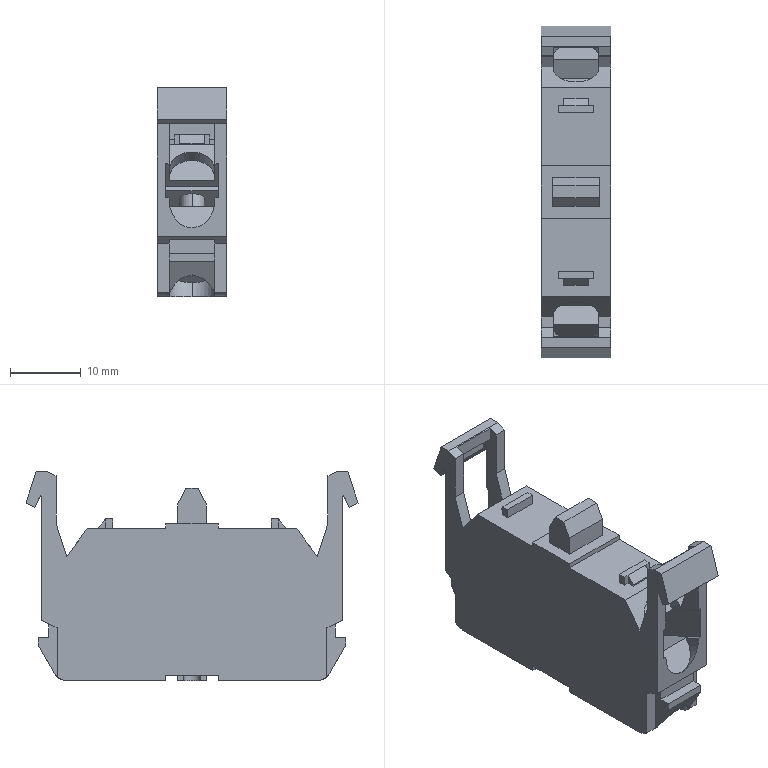Part | STEP file | A22NZ_S_G1[] | 1 solid | 189 faces | box 9.9 x 47 x 29.6 mm | volume 7656 mm3 | plane 160 | cylinder 29 | commonest cylinder face diameters 6.5 x6 3.5 x4 4 x4 5.8 x4 6 x4 6.4 x4